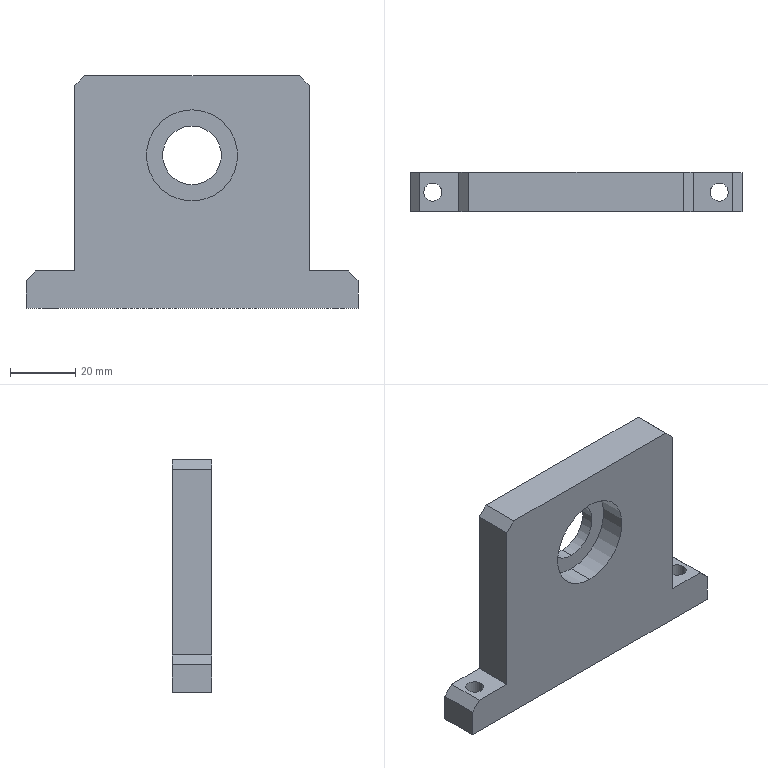Part | SolidWorks | features BaseBody 1 | 1 solid | 23 faces | box 102 x 12 x 71.5 mm | volume 59210 mm3 | plane 15 | cylinder 8 | commonest cylinder face diameters 5.5 x4 18 x2 28 x2
STEP:
#1=CARTESIAN_POINT('',(1.,-295.,36.5));
#2=VERTEX_POINT('',#1);
#3=CARTESIAN_POINT('',(1.,-295.,54.5));
#4=VERTEX_POINT('',#3);
#5=CARTESIAN_POINT('',(1.,-295.,45.5));
#6=DIRECTION('',(0.,1.,0.));
#7=DIRECTION('',(0.,0.,-1.));
#8=AXIS2_PLACEMENT_3D('',#5,#6,#7);
#9=CIRCLE('',#8,9.);
#10=EDGE_CURVE('',#2,#4,#9,.T.);
#11=ORIENTED_EDGE('',*,*,#10,.T.);
#12=CARTESIAN_POINT('',(1.,-299.,54.5));
#13=VERTEX_POINT('',#12);
#14=CARTESIAN_POINT('',(1.,-295.,54.5));
#15=DIRECTION('',(0.,-1.,0.));
#16=VECTOR('',#15,1000.);
#17=LINE('',#14,#16);
#18=EDGE_CURVE('',#4,#13,#17,.T.);
#19=ORIENTED_EDGE('',*,*,#18,.T.);
#20=CARTESIAN_POINT('',(1.,-299.,36.5));
#21=VERTEX_POINT('',#20);
#22=CARTESIAN_POINT('',(1.,-299.,45.5));
#23=DIRECTION('',(0.,1.,0.));
#24=DIRECTION('',(0.,0.,-1.));
#25=AXIS2_PLACEMENT_3D('',#22,#23,#24);
#26=CIRCLE('',#25,9.);
#27=EDGE_CURVE('',#21,#13,#26,.T.);
#28=ORIENTED_EDGE('',*,*,#27,.F.);
#29=CARTESIAN_POINT('',(1.,-295.,36.5));
#30=DIRECTION('',(0.,-1.,0.));
#31=VECTOR('',#30,1000.);
#32=LINE('',#29,#31);
#33=EDGE_CURVE('',#2,#21,#32,.T.);
#34=ORIENTED_EDGE('',*,*,#33,.F.);
#35=EDGE_LOOP('',(#11,#19,#28,#34));
#36=FACE_OUTER_BOUND('',#35,.T.);
#37=CARTESIAN_POINT('',(1.,-295.,45.5));
#38=DIRECTION('',(0.,-1.,0.));
#39=DIRECTION('',(0.,0.,-1.));
#40=AXIS2_PLACEMENT_3D('',#37,#38,#39);
#41=CYLINDRICAL_SURFACE('',#40,9.);
#42=ADVANCED_FACE('',(#36),#41,.F.);
#43=CARTESIAN_POINT('',(42.25,-301.,-1.5));
#44=VERTEX_POINT('',#43);
#45=CARTESIAN_POINT('',(47.75,-301.,-1.5));
#46=VERTEX_POINT('',#45);
#47=CARTESIAN_POINT('',(45.,-301.,-1.5));
#48=DIRECTION('',(0.,0.,1.));
#49=DIRECTION('',(1.,0.,0.));
#50=AXIS2_PLACEMENT_3D('',#47,#48,#49);
#51=CIRCLE('',#50,2.75);
#52=EDGE_CURVE('',#44,#46,#51,.T.);
#53=ORIENTED_EDGE('',*,*,#52,.F.);
#54=CARTESIAN_POINT('',(42.25,-301.,10.));
#55=VERTEX_POINT('',#54);
#56=CARTESIAN_POINT('',(42.25,-301.,0.));
#57=DIRECTION('',(0.,0.,1.));
#58=VECTOR('',#57,1000.);
#59=LINE('',#56,#58);
#60=EDGE_CURVE('',#44,#55,#59,.T.);
#61=ORIENTED_EDGE('',*,*,#60,.T.);
#62=CARTESIAN_POINT('',(47.75,-301.,10.));
#63=VERTEX_POINT('',#62);
#64=CARTESIAN_POINT('',(45.,-301.,10.));
#65=DIRECTION('',(0.,0.,1.));
#66=DIRECTION('',(1.,0.,0.));
#67=AXIS2_PLACEMENT_3D('',#64,#65,#66);
#68=CIRCLE('',#67,2.75);
#69=EDGE_CURVE('',#55,#63,#68,.T.);
#70=ORIENTED_EDGE('',*,*,#69,.T.);
#71=CARTESIAN_POINT('',(47.75,-301.,0.));
#72=DIRECTION('',(0.,0.,1.));
#73=VECTOR('',#72,1000.);
#74=LINE('',#71,#73);
#75=EDGE_CURVE('',#46,#63,#74,.T.);
#76=ORIENTED_EDGE('',*,*,#75,.F.);
#77=EDGE_LOOP('',(#53,#61,#70,#76));
#78=FACE_OUTER_BOUND('',#77,.T.);
#79=CARTESIAN_POINT('',(45.,-301.,0.));
#80=DIRECTION('',(0.,0.,1.));
#81=DIRECTION('',(1.,0.,0.));
#82=AXIS2_PLACEMENT_3D('',#79,#80,#81);
#83=CYLINDRICAL_SURFACE('',#82,2.75);
#84=ADVANCED_FACE('',(#78),#83,.F.);
#85=CARTESIAN_POINT('',(-45.75,-301.,-1.5));
#86=VERTEX_POINT('',#85);
#87=CARTESIAN_POINT('',(-40.25,-301.,-1.5));
#88=VERTEX_POINT('',#87);
#89=CARTESIAN_POINT('',(-43.,-301.,-1.5));
#90=DIRECTION('',(0.,0.,1.));
#91=DIRECTION('',(1.,0.,0.));
#92=AXIS2_PLACEMENT_3D('',#89,#90,#91);
#93=CIRCLE('',#92,2.75);
#94=EDGE_CURVE('',#86,#88,#93,.T.);
#95=ORIENTED_EDGE('',*,*,#94,.F.);
#96=CARTESIAN_POINT('',(-45.75,-301.,10.));
#97=VERTEX_POINT('',#96);
#98=CARTESIAN_POINT('',(-45.75,-301.,0.));
#99=DIRECTION('',(0.,0.,1.));
#100=VECTOR('',#99,1000.);
#101=LINE('',#98,#100);
#102=EDGE_CURVE('',#86,#97,#101,.T.);
#103=ORIENTED_EDGE('',*,*,#102,.T.);
#104=CARTESIAN_POINT('',(-40.25,-301.,10.));
#105=VERTEX_POINT('',#104);
#106=CARTESIAN_POINT('',(-43.,-301.,10.));
#107=DIRECTION('',(0.,0.,1.));
#108=DIRECTION('',(1.,0.,0.));
#109=AXIS2_PLACEMENT_3D('',#106,#107,#108);
#110=CIRCLE('',#109,2.75);
#111=EDGE_CURVE('',#97,#105,#110,.T.);
#112=ORIENTED_EDGE('',*,*,#111,.T.);
#113=CARTESIAN_POINT('',(-40.25,-301.,0.));
#114=DIRECTION('',(0.,0.,1.));
#115=VECTOR('',#114,1000.);
#116=LINE('',#113,#115);
#117=EDGE_CURVE('',#88,#105,#116,.T.);
#118=ORIENTED_EDGE('',*,*,#117,.F.);
#119=EDGE_LOOP('',(#95,#103,#112,#118));
#120=FACE_OUTER_BOUND('',#119,.T.);
#121=CARTESIAN_POINT('',(-43.,-301.,0.));
#122=DIRECTION('',(0.,0.,1.));
#123=DIRECTION('',(1.,0.,0.));
#124=AXIS2_PLACEMENT_3D('',#121,#122,#123);
#125=CYLINDRICAL_SURFACE('',#124,2.75);
#126=ADVANCED_FACE('',(#120),#125,.F.);
#127=CARTESIAN_POINT('',(1.,-299.,59.5));
#128=VERTEX_POINT('',#127);
#129=CARTESIAN_POINT('',(1.,-299.,31.5));
#130=VERTEX_POINT('',#129);
#131=CARTESIAN_POINT('',(1.,-299.,45.5));
#132=DIRECTION('',(0.,-1.,0.));
#133=DIRECTION('',(0.,0.,-1.));
#134=AXIS2_PLACEMENT_3D('',#131,#132,#133);
#135=CIRCLE('',#134,14.);
#136=EDGE_CURVE('',#128,#130,#135,.T.);
#137=ORIENTED_EDGE('',*,*,#136,.F.);
#138=CARTESIAN_POINT('',(1.,-307.,59.5));
#139=VERTEX_POINT('',#138);
#140=CARTESIAN_POINT('',(1.,-299.,59.5));
#141=DIRECTION('',(0.,-1.,0.));
#142=VECTOR('',#141,1000.);
#143=LINE('',#140,#142);
#144=EDGE_CURVE('',#128,#139,#143,.T.);
#145=ORIENTED_EDGE('',*,*,#144,.T.);
#146=CARTESIAN_POINT('',(1.,-307.,31.5));
#147=VERTEX_POINT('',#146);
#148=CARTESIAN_POINT('',(1.,-307.,45.5));
#149=DIRECTION('',(0.,-1.,0.));
#150=DIRECTION('',(0.,0.,-1.));
#151=AXIS2_PLACEMENT_3D('',#148,#149,#150);
#152=CIRCLE('',#151,14.);
#153=EDGE_CURVE('',#139,#147,#152,.T.);
#154=ORIENTED_EDGE('',*,*,#153,.T.);
#155=CARTESIAN_POINT('',(1.,-299.,31.5));
#156=DIRECTION('',(0.,-1.,0.));
#157=VECTOR('',#156,1000.);
#158=LINE('',#155,#157);
#159=EDGE_CURVE('',#130,#147,#158,.T.);
#160=ORIENTED_EDGE('',*,*,#159,.F.);
#161=EDGE_LOOP('',(#137,#145,#154,#160));
#162=FACE_OUTER_BOUND('',#161,.T.);
#163=CARTESIAN_POINT('',(1.,-299.,45.5));
#164=DIRECTION('',(0.,-1.,0.));
#165=DIRECTION('',(0.,0.,-1.));
#166=AXIS2_PLACEMENT_3D('',#163,#164,#165);
#167=CYLINDRICAL_SURFACE('',#166,14.);
#168=ADVANCED_FACE('',(#162),#167,.F.);
#169=CARTESIAN_POINT('',(37.,-295.,67.));
#170=VERTEX_POINT('',#169);
#171=CARTESIAN_POINT('',(34.,-295.,70.));
#172=VERTEX_POINT('',#171);
#173=CARTESIAN_POINT('',(37.,-295.,67.));
#174=DIRECTION('',(-0.7071,0.,0.7071));
#175=VECTOR('',#174,1000.);
#176=LINE('',#173,#175);
#177=EDGE_CURVE('',#170,#172,#176,.T.);
#178=ORIENTED_EDGE('',*,*,#177,.F.);
#179=CARTESIAN_POINT('',(37.,-295.,10.));
#180=VERTEX_POINT('',#179);
#181=CARTESIAN_POINT('',(37.,-295.,70.));
#182=DIRECTION('',(0.,0.,1.));
#183=VECTOR('',#182,1000.);
#184=LINE('',#181,#183);
#185=EDGE_CURVE('',#180,#170,#184,.T.);
#186=ORIENTED_EDGE('',*,*,#185,.F.);
#187=CARTESIAN_POINT('',(49.,-295.,10.));
#188=VERTEX_POINT('',#187);
#189=CARTESIAN_POINT('',(52.,-295.,10.));
#190=DIRECTION('',(-1.,0.,0.));
#191=VECTOR('',#190,1000.);
#192=LINE('',#189,#191);
#193=EDGE_CURVE('',#188,#180,#192,.T.);
#194=ORIENTED_EDGE('',*,*,#193,.F.);
#195=CARTESIAN_POINT('',(52.,-295.,7.));
#196=VERTEX_POINT('',#195);
#197=CARTESIAN_POINT('',(52.,-295.,7.));
#198=DIRECTION('',(-0.7071,0.,0.7071));
#199=VECTOR('',#198,1000.);
#200=LINE('',#197,#199);
#201=EDGE_CURVE('',#196,#188,#200,.T.);
#202=ORIENTED_EDGE('',*,*,#201,.F.);
#203=CARTESIAN_POINT('',(52.,-295.,-1.5));
#204=VERTEX_POINT('',#203);
#205=CARTESIAN_POINT('',(52.,-295.,70.));
#206=DIRECTION('',(0.,0.,1.));
#207=VECTOR('',#206,1000.);
#208=LINE('',#205,#207);
#209=EDGE_CURVE('',#204,#196,#208,.T.);
#210=ORIENTED_EDGE('',*,*,#209,.F.);
#211=CARTESIAN_POINT('',(-50.,-295.,-1.5));
#212=VERTEX_POINT('',#211);
#213=CARTESIAN_POINT('',(52.,-295.,-1.5));
#214=DIRECTION('',(1.,0.,0.));
#215=VECTOR('',#214,1000.);
#216=LINE('',#213,#215);
#217=EDGE_CURVE('',#212,#204,#216,.T.);
#218=ORIENTED_EDGE('',*,*,#217,.F.);
#219=CARTESIAN_POINT('',(-50.,-295.,7.));
#220=VERTEX_POINT('',#219);
#221=CARTESIAN_POINT('',(-50.,-295.,70.));
#222=DIRECTION('',(0.,0.,-1.));
#223=VECTOR('',#222,1000.);
#224=LINE('',#221,#223);
#225=EDGE_CURVE('',#220,#212,#224,.T.);
#226=ORIENTED_EDGE('',*,*,#225,.F.);
#227=CARTESIAN_POINT('',(-47.,-295.,10.));
#228=VERTEX_POINT('',#227);
#229=CARTESIAN_POINT('',(-47.,-295.,10.));
#230=DIRECTION('',(-0.7071,0.,-0.7071));
#231=VECTOR('',#230,1000.);
#232=LINE('',#229,#231);
#233=EDGE_CURVE('',#228,#220,#232,.T.);
#234=ORIENTED_EDGE('',*,*,#233,.F.);
#235=CARTESIAN_POINT('',(-35.,-295.,10.));
#236=VERTEX_POINT('',#235);
#237=CARTESIAN_POINT('',(52.,-295.,10.));
#238=DIRECTION('',(-1.,0.,0.));
#239=VECTOR('',#238,1000.);
#240=LINE('',#237,#239);
#241=EDGE_CURVE('',#236,#228,#240,.T.);
#242=ORIENTED_EDGE('',*,*,#241,.F.);
#243=CARTESIAN_POINT('',(-35.,-295.,67.));
#244=VERTEX_POINT('',#243);
#245=CARTESIAN_POINT('',(-35.,-295.,70.));
#246=DIRECTION('',(0.,0.,-1.));
#247=VECTOR('',#246,1000.);
#248=LINE('',#245,#247);
#249=EDGE_CURVE('',#244,#236,#248,.T.);
#250=ORIENTED_EDGE('',*,*,#249,.F.);
#251=CARTESIAN_POINT('',(-32.,-295.,70.));
#252=VERTEX_POINT('',#251);
#253=CARTESIAN_POINT('',(-32.,-295.,70.));
#254=DIRECTION('',(-0.7071,0.,-0.7071));
#255=VECTOR('',#254,1000.);
#256=LINE('',#253,#255);
#257=EDGE_CURVE('',#252,#244,#256,.T.);
#258=ORIENTED_EDGE('',*,*,#257,.F.);
#259=CARTESIAN_POINT('',(52.,-295.,70.));
#260=DIRECTION('',(-1.,0.,0.));
#261=VECTOR('',#260,1000.);
#262=LINE('',#259,#261);
#263=EDGE_CURVE('',#172,#252,#262,.T.);
#264=ORIENTED_EDGE('',*,*,#263,.F.);
#265=EDGE_LOOP('',(#178,#186,#194,#202,#210,#218,#226,#234,#242,#250,#258,#264));
#266=FACE_OUTER_BOUND('',#265,.T.);
#267=ORIENTED_EDGE('',*,*,#10,.F.);
#268=CARTESIAN_POINT('',(1.,-295.,45.5));
#269=DIRECTION('',(0.,1.,0.));
#270=DIRECTION('',(0.,0.,-1.));
#271=AXIS2_PLACEMENT_3D('',#268,#269,#270);
#272=CIRCLE('',#271,9.);
#273=EDGE_CURVE('',#4,#2,#272,.T.);
#274=ORIENTED_EDGE('',*,*,#273,.F.);
#275=EDGE_LOOP('',(#267,#274));
#276=FACE_BOUND('',#275,.T.);
#277=CARTESIAN_POINT('',(52.,-295.,70.));
#278=DIRECTION('',(0.,-1.,0.));
#279=DIRECTION('',(0.,0.,-1.));
#280=AXIS2_PLACEMENT_3D('',#277,#278,#279);
#281=PLANE('',#280);
#282=ADVANCED_FACE('',(#266,#276),#281,.F.);
#283=ORIENTED_EDGE('',*,*,#263,.T.);
#284=CARTESIAN_POINT('',(-32.,-307.,70.));
#285=VERTEX_POINT('',#284);
#286=CARTESIAN_POINT('',(-32.,0.,70.));
#287=DIRECTION('',(0.,-1.,0.));
#288=VECTOR('',#287,1000.);
#289=LINE('',#286,#288);
#290=EDGE_CURVE('',#252,#285,#289,.T.);
#291=ORIENTED_EDGE('',*,*,#290,.T.);
#292=CARTESIAN_POINT('',(34.,-307.,70.));
#293=VERTEX_POINT('',#292);
#294=CARTESIAN_POINT('',(0.,-307.,70.));
#295=DIRECTION('',(1.,0.,0.));
#296=VECTOR('',#295,1000.);
#297=LINE('',#294,#296);
#298=EDGE_CURVE('',#285,#293,#297,.T.);
#299=ORIENTED_EDGE('',*,*,#298,.T.);
#300=CARTESIAN_POINT('',(34.,0.,70.));
#301=DIRECTION('',(0.,1.,0.));
#302=VECTOR('',#301,1000.);
#303=LINE('',#300,#302);
#304=EDGE_CURVE('',#293,#172,#303,.T.);
#305=ORIENTED_EDGE('',*,*,#304,.T.);
#306=EDGE_LOOP('',(#283,#291,#299,#305));
#307=FACE_OUTER_BOUND('',#306,.T.);
#308=CARTESIAN_POINT('',(0.,0.,70.));
#309=DIRECTION('',(0.,0.,1.));
#310=DIRECTION('',(1.,0.,0.));
#311=AXIS2_PLACEMENT_3D('',#308,#309,#310);
#312=PLANE('',#311);
#313=ADVANCED_FACE('',(#307),#312,.T.);
#314=CARTESIAN_POINT('',(37.,-307.,67.));
#315=VERTEX_POINT('',#314);
#316=CARTESIAN_POINT('',(37.,-307.,67.));
#317=DIRECTION('',(0.7071,0.,-0.7071));
#318=VECTOR('',#317,1000.);
#319=LINE('',#316,#318);
#320=EDGE_CURVE('',#293,#315,#319,.T.);
#321=ORIENTED_EDGE('',*,*,#320,.T.);
#322=CARTESIAN_POINT('',(37.,-295.,67.));
#323=DIRECTION('',(0.,1.,0.));
#324=VECTOR('',#323,1000.);
#325=LINE('',#322,#324);
#326=EDGE_CURVE('',#315,#170,#325,.T.);
#327=ORIENTED_EDGE('',*,*,#326,.T.);
#328=ORIENTED_EDGE('',*,*,#177,.T.);
#329=ORIENTED_EDGE('',*,*,#304,.F.);
#330=EDGE_LOOP('',(#321,#327,#328,#329));
#331=FACE_OUTER_BOUND('',#330,.T.);
#332=CARTESIAN_POINT('',(37.,-295.,67.));
#333=DIRECTION('',(0.7071,0.,0.7071));
#334=DIRECTION('',(0.7071,0.,-0.7071));
#335=AXIS2_PLACEMENT_3D('',#332,#333,#334);
#336=PLANE('',#335);
#337=ADVANCED_FACE('',(#331),#336,.T.);
#338=ORIENTED_EDGE('',*,*,#326,.F.);
#339=CARTESIAN_POINT('',(37.,-307.,10.));
#340=VERTEX_POINT('',#339);
#341=CARTESIAN_POINT('',(37.,-307.,70.));
#342=DIRECTION('',(0.,0.,1.));
#343=VECTOR('',#342,1000.);
#344=LINE('',#341,#343);
#345=EDGE_CURVE('',#340,#315,#344,.T.);
#346=ORIENTED_EDGE('',*,*,#345,.F.);
#347=CARTESIAN_POINT('',(37.,-295.,10.));
#348=DIRECTION('',(0.,-1.,0.));
#349=VECTOR('',#348,1000.);
#350=LINE('',#347,#349);
#351=EDGE_CURVE('',#180,#340,#350,.T.);
#352=ORIENTED_EDGE('',*,*,#351,.F.);
#353=ORIENTED_EDGE('',*,*,#185,.T.);
#354=EDGE_LOOP('',(#338,#346,#352,#353));
#355=FACE_OUTER_BOUND('',#354,.T.);
#356=CARTESIAN_POINT('',(37.,-295.,70.));
#357=DIRECTION('',(-1.,0.,0.));
#358=DIRECTION('',(0.,0.,1.));
#359=AXIS2_PLACEMENT_3D('',#356,#357,#358);
#360=PLANE('',#359);
#361=ADVANCED_FACE('',(#355),#360,.F.);
#362=CARTESIAN_POINT('',(49.,-307.,10.));
#363=VERTEX_POINT('',#362);
#364=CARTESIAN_POINT('',(49.,-295.,10.));
#365=DIRECTION('',(0.,-1.,0.));
#366=VECTOR('',#365,1000.);
#367=LINE('',#364,#366);
#368=EDGE_CURVE('',#188,#363,#367,.T.);
#369=ORIENTED_EDGE('',*,*,#368,.F.);
#370=ORIENTED_EDGE('',*,*,#193,.T.);
#371=ORIENTED_EDGE('',*,*,#351,.T.);
#372=CARTESIAN_POINT('',(52.,-307.,10.));
#373=DIRECTION('',(-1.,0.,0.));
#374=VECTOR('',#373,1000.);
#375=LINE('',#372,#374);
#376=EDGE_CURVE('',#363,#340,#375,.T.);
#377=ORIENTED_EDGE('',*,*,#376,.F.);
#378=EDGE_LOOP('',(#369,#370,#371,#377));
#379=FACE_OUTER_BOUND('',#378,.T.);
#380=CARTESIAN_POINT('',(45.,-301.,10.));
#381=DIRECTION('',(0.,0.,1.));
#382=DIRECTION('',(1.,0.,0.));
#383=AXIS2_PLACEMENT_3D('',#380,#381,#382);
#384=CIRCLE('',#383,2.75);
#385=EDGE_CURVE('',#63,#55,#384,.T.);
#386=ORIENTED_EDGE('',*,*,#385,.F.);
#387=ORIENTED_EDGE('',*,*,#69,.F.);
#388=EDGE_LOOP('',(#386,#387));
#389=FACE_BOUND('',#388,.T.);
#390=CARTESIAN_POINT('',(52.,-295.,10.));
#391=DIRECTION('',(0.,0.,-1.));
#392=DIRECTION('',(-1.,0.,0.));
#393=AXIS2_PLACEMENT_3D('',#390,#391,#392);
#394=PLANE('',#393);
#395=ADVANCED_FACE('',(#379,#389),#394,.F.);
#396=ORIENTED_EDGE('',*,*,#368,.T.);
#397=CARTESIAN_POINT('',(52.,-307.,7.));
#398=VERTEX_POINT('',#397);
#399=CARTESIAN_POINT('',(52.,-307.,7.));
#400=DIRECTION('',(-0.7071,0.,0.7071));
#401=VECTOR('',#400,1000.);
#402=LINE('',#399,#401);
#403=EDGE_CURVE('',#398,#363,#402,.T.);
#404=ORIENTED_EDGE('',*,*,#403,.F.);
#405=CARTESIAN_POINT('',(52.,-307.,7.));
#406=DIRECTION('',(0.,-1.,0.));
#407=VECTOR('',#406,1000.);
#408=LINE('',#405,#407);
#409=EDGE_CURVE('',#196,#398,#408,.T.);
#410=ORIENTED_EDGE('',*,*,#409,.F.);
#411=ORIENTED_EDGE('',*,*,#201,.T.);
#412=EDGE_LOOP('',(#396,#404,#410,#411));
#413=FACE_OUTER_BOUND('',#412,.T.);
#414=CARTESIAN_POINT('',(52.,-307.,7.));
#415=DIRECTION('',(-0.7071,0.,-0.7071));
#416=DIRECTION('',(-0.7071,0.,0.7071));
#417=AXIS2_PLACEMENT_3D('',#414,#415,#416);
#418=PLANE('',#417);
#419=ADVANCED_FACE('',(#413),#418,.F.);
#420=ORIENTED_EDGE('',*,*,#409,.T.);
#421=CARTESIAN_POINT('',(52.,-307.,-1.5));
#422=VERTEX_POINT('',#421);
#423=CARTESIAN_POINT('',(52.,-307.,70.));
#424=DIRECTION('',(0.,0.,1.));
#425=VECTOR('',#424,1000.);
#426=LINE('',#423,#425);
#427=EDGE_CURVE('',#422,#398,#426,.T.);
#428=ORIENTED_EDGE('',*,*,#427,.F.);
#429=CARTESIAN_POINT('',(52.,-307.,-1.5));
#430=DIRECTION('',(0.,-1.,0.));
#431=VECTOR('',#430,1000.);
#432=LINE('',#429,#431);
#433=EDGE_CURVE('',#204,#422,#432,.T.);
#434=ORIENTED_EDGE('',*,*,#433,.F.);
#435=ORIENTED_EDGE('',*,*,#209,.T.);
#436=EDGE_LOOP('',(#420,#428,#434,#435));
#437=FACE_OUTER_BOUND('',#436,.T.);
#438=CARTESIAN_POINT('',(52.,-307.,70.));
#439=DIRECTION('',(-1.,0.,0.));
#440=DIRECTION('',(0.,0.,1.));
#441=AXIS2_PLACEMENT_3D('',#438,#439,#440);
#442=PLANE('',#441);
#443=ADVANCED_FACE('',(#437),#442,.F.);
#444=CARTESIAN_POINT('',(45.,-301.,-1.5));
#445=DIRECTION('',(0.,0.,1.));
#446=DIRECTION('',(1.,0.,0.));
#447=AXIS2_PLACEMENT_3D('',#444,#445,#446);
#448=CIRCLE('',#447,2.75);
#449=EDGE_CURVE('',#46,#44,#448,.T.);
#450=ORIENTED_EDGE('',*,*,#449,.T.);
#451=ORIENTED_EDGE('',*,*,#52,.T.);
#452=EDGE_LOOP('',(#450,#451));
#453=FACE_BOUND('',#452,.T.);
#454=CARTESIAN_POINT('',(-50.,-307.,-1.5));
#455=VERTEX_POINT('',#454);
#456=CARTESIAN_POINT('',(0.,-307.,-1.5));
#457=DIRECTION('',(-1.,0.,0.));
#458=VECTOR('',#457,1000.);
#459=LINE('',#456,#458);
#460=EDGE_CURVE('',#422,#455,#459,.T.);
#461=ORIENTED_EDGE('',*,*,#460,.T.);
#462=CARTESIAN_POINT('',(-50.,0.,-1.5));
#463=DIRECTION('',(0.,1.,0.));
#464=VECTOR('',#463,1000.);
#465=LINE('',#462,#464);
#466=EDGE_CURVE('',#455,#212,#465,.T.);
#467=ORIENTED_EDGE('',*,*,#466,.T.);
#468=ORIENTED_EDGE('',*,*,#217,.T.);
#469=ORIENTED_EDGE('',*,*,#433,.T.);
#470=EDGE_LOOP('',(#461,#467,#468,#469));
#471=FACE_OUTER_BOUND('',#470,.T.);
#472=CARTESIAN_POINT('',(-43.,-301.,-1.5));
#473=DIRECTION('',(0.,0.,1.));
#474=DIRECTION('',(1.,0.,0.));
#475=AXIS2_PLACEMENT_3D('',#472,#473,#474);
#476=CIRCLE('',#475,2.75);
#477=EDGE_CURVE('',#88,#86,#476,.T.);
#478=ORIENTED_EDGE('',*,*,#477,.T.);
#479=ORIENTED_EDGE('',*,*,#94,.T.);
#480=EDGE_LOOP('',(#478,#479));
#481=FACE_BOUND('',#480,.T.);
#482=CARTESIAN_POINT('',(0.,0.,-1.5));
#483=DIRECTION('',(0.,0.,-1.));
#484=DIRECTION('',(-1.,0.,0.));
#485=AXIS2_PLACEMENT_3D('',#482,#483,#484);
#486=PLANE('',#485);
#487=ADVANCED_FACE('',(#453,#471,#481),#486,.T.);
#488=CARTESIAN_POINT('',(-50.,-307.,7.));
#489=VERTEX_POINT('',#488);
#490=CARTESIAN_POINT('',(-50.,-307.,7.));
#491=DIRECTION('',(0.,-1.,0.));
#492=VECTOR('',#491,1000.);
#493=LINE('',#490,#492);
#494=EDGE_CURVE('',#220,#489,#493,.T.);
#495=ORIENTED_EDGE('',*,*,#494,.F.);
#496=ORIENTED_EDGE('',*,*,#225,.T.);
#497=ORIENTED_EDGE('',*,*,#466,.F.);
#498=CARTESIAN_POINT('',(-50.,-307.,70.));
#499=DIRECTION('',(0.,0.,-1.));
#500=VECTOR('',#499,1000.);
#501=LINE('',#498,#500);
#502=EDGE_CURVE('',#489,#455,#501,.T.);
#503=ORIENTED_EDGE('',*,*,#502,.F.);
#504=EDGE_LOOP('',(#495,#496,#497,#503));
#505=FACE_OUTER_BOUND('',#504,.T.);
#506=CARTESIAN_POINT('',(-50.,-307.,70.));
#507=DIRECTION('',(1.,0.,0.));
#508=DIRECTION('',(0.,0.,-1.));
#509=AXIS2_PLACEMENT_3D('',#506,#507,#508);
#510=PLANE('',#509);
#511=ADVANCED_FACE('',(#505),#510,.F.);
#512=ORIENTED_EDGE('',*,*,#494,.T.);
#513=CARTESIAN_POINT('',(-47.,-307.,10.));
#514=VERTEX_POINT('',#513);
#515=CARTESIAN_POINT('',(-47.,-307.,10.));
#516=DIRECTION('',(-0.7071,0.,-0.7071));
#517=VECTOR('',#516,1000.);
#518=LINE('',#515,#517);
#519=EDGE_CURVE('',#514,#489,#518,.T.);
#520=ORIENTED_EDGE('',*,*,#519,.F.);
#521=CARTESIAN_POINT('',(-47.,-295.,10.));
#522=DIRECTION('',(0.,-1.,0.));
#523=VECTOR('',#522,1000.);
#524=LINE('',#521,#523);
#525=EDGE_CURVE('',#228,#514,#524,.T.);
#526=ORIENTED_EDGE('',*,*,#525,.F.);
#527=ORIENTED_EDGE('',*,*,#233,.T.);
#528=EDGE_LOOP('',(#512,#520,#526,#527));
#529=FACE_OUTER_BOUND('',#528,.T.);
#530=CARTESIAN_POINT('',(-47.,-295.,10.));
#531=DIRECTION('',(0.7071,0.,-0.7071));
#532=DIRECTION('',(-0.7071,0.,-0.7071));
#533=AXIS2_PLACEMENT_3D('',#530,#531,#532);
#534=PLANE('',#533);
#535=ADVANCED_FACE('',(#529),#534,.F.);
#536=ORIENTED_EDGE('',*,*,#525,.T.);
#537=CARTESIAN_POINT('',(-35.,-307.,10.));
#538=VERTEX_POINT('',#537);
#539=CARTESIAN_POINT('',(-50.,-307.,10.));
#540=DIRECTION('',(-1.,0.,0.));
#541=VECTOR('',#540,1000.);
#542=LINE('',#539,#541);
#543=EDGE_CURVE('',#538,#514,#542,.T.);
#544=ORIENTED_EDGE('',*,*,#543,.F.);
#545=CARTESIAN_POINT('',(-35.,-295.,10.));
#546=DIRECTION('',(0.,-1.,0.));
#547=VECTOR('',#546,1000.);
#548=LINE('',#545,#547);
#549=EDGE_CURVE('',#236,#538,#548,.T.);
#550=ORIENTED_EDGE('',*,*,#549,.F.);
#551=ORIENTED_EDGE('',*,*,#241,.T.);
#552=EDGE_LOOP('',(#536,#544,#550,#551));
#553=FACE_OUTER_BOUND('',#552,.T.);
#554=CARTESIAN_POINT('',(-43.,-301.,10.));
#555=DIRECTION('',(0.,0.,1.));
#556=DIRECTION('',(1.,0.,0.));
#557=AXIS2_PLACEMENT_3D('',#554,#555,#556);
#558=CIRCLE('',#557,2.75);
#559=EDGE_CURVE('',#105,#97,#558,.T.);
#560=ORIENTED_EDGE('',*,*,#559,.F.);
#561=ORIENTED_EDGE('',*,*,#111,.F.);
#562=EDGE_LOOP('',(#560,#561));
#563=FACE_BOUND('',#562,.T.);
#564=CARTESIAN_POINT('',(-50.,-295.,10.));
#565=DIRECTION('',(0.,0.,-1.));
#566=DIRECTION('',(-1.,0.,0.));
#567=AXIS2_PLACEMENT_3D('',#564,#565,#566);
#568=PLANE('',#567);
#569=ADVANCED_FACE('',(#553,#563),#568,.F.);
#570=CARTESIAN_POINT('',(-35.,-307.,67.));
#571=VERTEX_POINT('',#570);
#572=CARTESIAN_POINT('',(-35.,-295.,67.));
#573=DIRECTION('',(0.,-1.,0.));
#574=VECTOR('',#573,1000.);
#575=LINE('',#572,#574);
#576=EDGE_CURVE('',#244,#571,#575,.T.);
#577=ORIENTED_EDGE('',*,*,#576,.F.);
#578=ORIENTED_EDGE('',*,*,#249,.T.);
#579=ORIENTED_EDGE('',*,*,#549,.T.);
#580=CARTESIAN_POINT('',(-35.,-307.,70.));
#581=DIRECTION('',(0.,0.,-1.));
#582=VECTOR('',#581,1000.);
#583=LINE('',#580,#582);
#584=EDGE_CURVE('',#571,#538,#583,.T.);
#585=ORIENTED_EDGE('',*,*,#584,.F.);
#586=EDGE_LOOP('',(#577,#578,#579,#585));
#587=FACE_OUTER_BOUND('',#586,.T.);
#588=CARTESIAN_POINT('',(-35.,-295.,70.));
#589=DIRECTION('',(1.,0.,0.));
#590=DIRECTION('',(0.,0.,-1.));
#591=AXIS2_PLACEMENT_3D('',#588,#589,#590);
#592=PLANE('',#591);
#593=ADVANCED_FACE('',(#587),#592,.F.);
#594=CARTESIAN_POINT('',(-32.,-307.,70.));
#595=DIRECTION('',(0.7071,0.,0.7071));
#596=VECTOR('',#595,1000.);
#597=LINE('',#594,#596);
#598=EDGE_CURVE('',#571,#285,#597,.T.);
#599=ORIENTED_EDGE('',*,*,#598,.T.);
#600=ORIENTED_EDGE('',*,*,#290,.F.);
#601=ORIENTED_EDGE('',*,*,#257,.T.);
#602=ORIENTED_EDGE('',*,*,#576,.T.);
#603=EDGE_LOOP('',(#599,#600,#601,#602));
#604=FACE_OUTER_BOUND('',#603,.T.);
#605=CARTESIAN_POINT('',(-32.,0.,70.));
#606=DIRECTION('',(-0.7071,0.,0.7071));
#607=DIRECTION('',(0.7071,0.,0.7071));
#608=AXIS2_PLACEMENT_3D('',#605,#606,#607);
#609=PLANE('',#608);
#610=ADVANCED_FACE('',(#604),#609,.T.);
#611=ORIENTED_EDGE('',*,*,#18,.F.);
#612=ORIENTED_EDGE('',*,*,#273,.T.);
#613=ORIENTED_EDGE('',*,*,#33,.T.);
#614=CARTESIAN_POINT('',(1.,-299.,45.5));
#615=DIRECTION('',(0.,1.,0.));
#616=DIRECTION('',(0.,0.,-1.));
#617=AXIS2_PLACEMENT_3D('',#614,#615,#616);
#618=CIRCLE('',#617,9.);
#619=EDGE_CURVE('',#13,#21,#618,.T.);
#620=ORIENTED_EDGE('',*,*,#619,.F.);
#621=EDGE_LOOP('',(#611,#612,#613,#620));
#622=FACE_OUTER_BOUND('',#621,.T.);
#623=CARTESIAN_POINT('',(1.,-295.,45.5));
#624=DIRECTION('',(0.,-1.,0.));
#625=DIRECTION('',(0.,0.,-1.));
#626=AXIS2_PLACEMENT_3D('',#623,#624,#625);
#627=CYLINDRICAL_SURFACE('',#626,9.);
#628=ADVANCED_FACE('',(#622),#627,.F.);
#629=ORIENTED_EDGE('',*,*,#320,.F.);
#630=ORIENTED_EDGE('',*,*,#298,.F.);
#631=ORIENTED_EDGE('',*,*,#598,.F.);
#632=ORIENTED_EDGE('',*,*,#584,.T.);
#633=ORIENTED_EDGE('',*,*,#543,.T.);
#634=ORIENTED_EDGE('',*,*,#519,.T.);
#635=ORIENTED_EDGE('',*,*,#502,.T.);
#636=ORIENTED_EDGE('',*,*,#460,.F.);
#637=ORIENTED_EDGE('',*,*,#427,.T.);
#638=ORIENTED_EDGE('',*,*,#403,.T.);
#639=ORIENTED_EDGE('',*,*,#376,.T.);
#640=ORIENTED_EDGE('',*,*,#345,.T.);
#641=EDGE_LOOP('',(#629,#630,#631,#632,#633,#634,#635,#636,#637,#638,#639,#640));
#642=FACE_OUTER_BOUND('',#641,.T.);
#643=CARTESIAN_POINT('',(1.,-307.,45.5));
#644=DIRECTION('',(0.,-1.,0.));
#645=DIRECTION('',(0.,0.,-1.));
#646=AXIS2_PLACEMENT_3D('',#643,#644,#645);
#647=CIRCLE('',#646,14.);
#648=EDGE_CURVE('',#147,#139,#647,.T.);
#649=ORIENTED_EDGE('',*,*,#648,.F.);
#650=ORIENTED_EDGE('',*,*,#153,.F.);
#651=EDGE_LOOP('',(#649,#650));
#652=FACE_BOUND('',#651,.T.);
#653=CARTESIAN_POINT('',(52.,-307.,70.));
#654=DIRECTION('',(0.,1.,0.));
#655=DIRECTION('',(0.,0.,1.));
#656=AXIS2_PLACEMENT_3D('',#653,#654,#655);
#657=PLANE('',#656);
#658=ADVANCED_FACE('',(#642,#652),#657,.F.);
#659=ORIENTED_EDGE('',*,*,#60,.F.);
#660=ORIENTED_EDGE('',*,*,#449,.F.);
#661=ORIENTED_EDGE('',*,*,#75,.T.);
#662=ORIENTED_EDGE('',*,*,#385,.T.);
#663=EDGE_LOOP('',(#659,#660,#661,#662));
#664=FACE_OUTER_BOUND('',#663,.T.);
#665=CARTESIAN_POINT('',(45.,-301.,0.));
#666=DIRECTION('',(0.,0.,1.));
#667=DIRECTION('',(1.,0.,0.));
#668=AXIS2_PLACEMENT_3D('',#665,#666,#667);
#669=CYLINDRICAL_SURFACE('',#668,2.75);
#670=ADVANCED_FACE('',(#664),#669,.F.);
#671=ORIENTED_EDGE('',*,*,#102,.F.);
#672=ORIENTED_EDGE('',*,*,#477,.F.);
#673=ORIENTED_EDGE('',*,*,#117,.T.);
#674=ORIENTED_EDGE('',*,*,#559,.T.);
#675=EDGE_LOOP('',(#671,#672,#673,#674));
#676=FACE_OUTER_BOUND('',#675,.T.);
#677=CARTESIAN_POINT('',(-43.,-301.,0.));
#678=DIRECTION('',(0.,0.,1.));
#679=DIRECTION('',(1.,0.,0.));
#680=AXIS2_PLACEMENT_3D('',#677,#678,#679);
#681=CYLINDRICAL_SURFACE('',#680,2.75);
#682=ADVANCED_FACE('',(#676),#681,.F.);
#683=CARTESIAN_POINT('',(1.,-299.,45.5));
#684=DIRECTION('',(0.,-1.,0.));
#685=DIRECTION('',(0.,0.,-1.));
#686=AXIS2_PLACEMENT_3D('',#683,#684,#685);
#687=CIRCLE('',#686,14.);
#688=EDGE_CURVE('',#130,#128,#687,.T.);
#689=ORIENTED_EDGE('',*,*,#688,.T.);
#690=ORIENTED_EDGE('',*,*,#136,.T.);
#691=EDGE_LOOP('',(#689,#690));
#692=FACE_OUTER_BOUND('',#691,.T.);
#693=ORIENTED_EDGE('',*,*,#27,.T.);
#694=ORIENTED_EDGE('',*,*,#619,.T.);
#695=EDGE_LOOP('',(#693,#694));
#696=FACE_BOUND('',#695,.T.);
#697=CARTESIAN_POINT('',(1.,-299.,45.5));
#698=DIRECTION('',(0.,-1.,0.));
#699=DIRECTION('',(0.,0.,-1.));
#700=AXIS2_PLACEMENT_3D('',#697,#698,#699);
#701=PLANE('',#700);
#702=ADVANCED_FACE('',(#692,#696),#701,.T.);
#703=ORIENTED_EDGE('',*,*,#144,.F.);
#704=ORIENTED_EDGE('',*,*,#688,.F.);
#705=ORIENTED_EDGE('',*,*,#159,.T.);
#706=ORIENTED_EDGE('',*,*,#648,.T.);
#707=EDGE_LOOP('',(#703,#704,#705,#706));
#708=FACE_OUTER_BOUND('',#707,.T.);
#709=CARTESIAN_POINT('',(1.,-299.,45.5));
#710=DIRECTION('',(0.,-1.,0.));
#711=DIRECTION('',(0.,0.,-1.));
#712=AXIS2_PLACEMENT_3D('',#709,#710,#711);
#713=CYLINDRICAL_SURFACE('',#712,14.);
#714=ADVANCED_FACE('',(#708),#713,.F.);
#715=CLOSED_SHELL('',(#42,#84,#126,#168,#282,#313,#337,#361,#395,#419,#443,#487,#511,#535,#569,#593,#610,#628,#658,#670,#682,#702,#714));
#716=MANIFOLD_SOLID_BREP('',#715);
#717=CARTESIAN_POINT('',(0.,0.,0.));
#718=DIRECTION('',(0.,0.,1.));
#719=DIRECTION('',(1.,0.,0.));
#720=AXIS2_PLACEMENT_3D('',#717,#718,#719);
#721=(LENGTH_UNIT()NAMED_UNIT(*)SI_UNIT(.MILLI.,.METRE.));
#722=UNCERTAINTY_MEASURE_WITH_UNIT(LENGTH_MEASURE(0.00001),#721,'','');
#723=(NAMED_UNIT(*)PLANE_ANGLE_UNIT()SI_UNIT($,.RADIAN.));
#724=(NAMED_UNIT(*)SI_UNIT($,.STERADIAN.)SOLID_ANGLE_UNIT());
#725=(GEOMETRIC_REPRESENTATION_CONTEXT(3)GLOBAL_UNCERTAINTY_ASSIGNED_CONTEXT((#722))GLOBAL_UNIT_ASSIGNED_CONTEXT((#721,#723,#724))REPRESENTATION_CONTEXT('',''));
#726=ADVANCED_BREP_SHAPE_REPRESENTATION('',(#716,#720),#725);